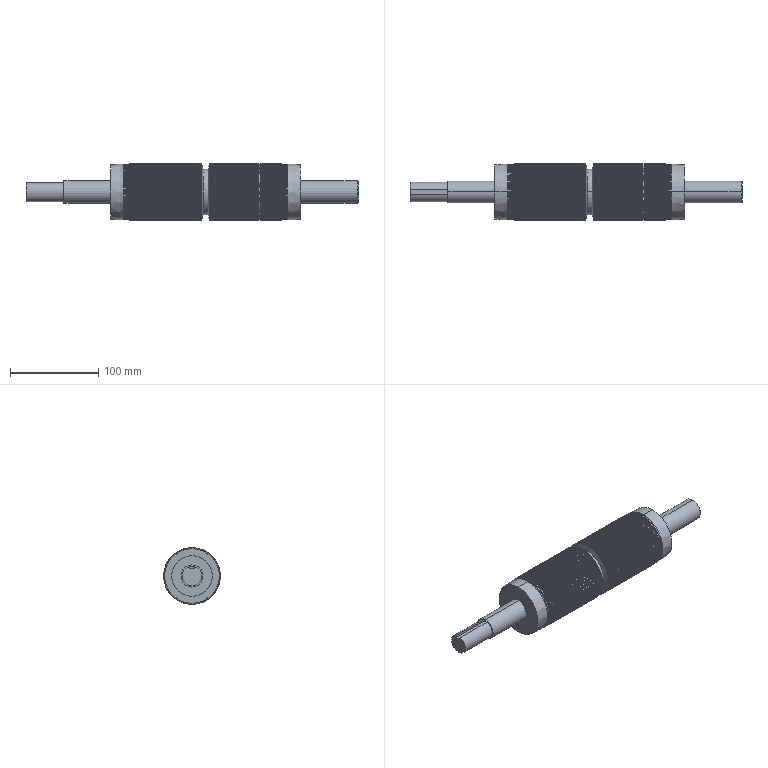Part | STEP file | MM-P46715-02_1 | 3 solids | 954 faces | box 375.959 x 63.996 x 63.999 mm | volume 524542 mm3 | plane 619 | cylinder 323 | cone 12 | commonest cylinder face diameters 64 x302 46 x8 25 x4 5 x2 22 x2 40 x2